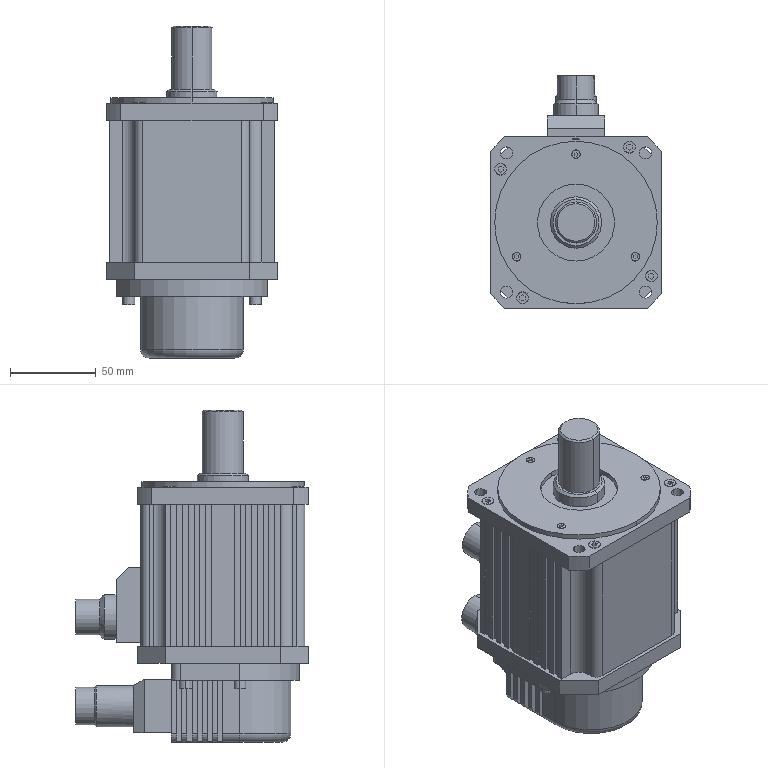Part | SolidWorks | features ICE 1, MBimport 1 | 1 solid | 422 faces | box 100 x 136 x 194 mm | volume 1174921 mm3 | plane 282 | cylinder 131 | cone 8 | torus 1 | commonest cylinder face diameters 7 x16 2.6 x8 3 x8 6.8 x8 6.937 x8 10 x8